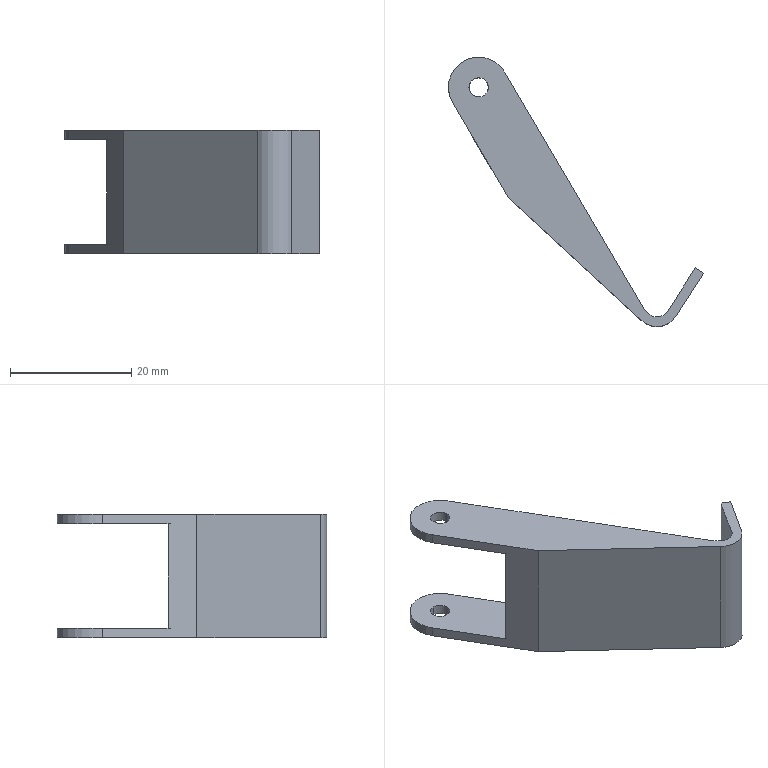Part | SolidWorks | features BaseBody 1 | 1 solid | 20 faces | box 42.12 x 44.482 x 20.4 mm | volume 2539 mm3 | plane 12 | cylinder 8 | commonest cylinder face diameters 3.2 x4 10 x2 4.14 x1 7.34 x1
STEP:
#1=CARTESIAN_POINT('',(2.549,31.982,8.6));
#2=VERTEX_POINT('',#1);
#3=CARTESIAN_POINT('',(-0.6512,31.982,8.6));
#4=VERTEX_POINT('',#3);
#5=CARTESIAN_POINT('',(0.9488,31.982,8.6));
#6=DIRECTION('',(0.,0.,-1.));
#7=DIRECTION('',(1.,0.,0.));
#8=AXIS2_PLACEMENT_3D('',#5,#6,#7);
#9=CIRCLE('',#8,1.6);
#10=EDGE_CURVE('',#2,#4,#9,.T.);
#11=ORIENTED_EDGE('',*,*,#10,.T.);
#12=CARTESIAN_POINT('',(-0.6512,31.982,10.2));
#13=VERTEX_POINT('',#12);
#14=CARTESIAN_POINT('',(-0.6512,31.982,8.6));
#15=DIRECTION('',(0.,0.,1.));
#16=VECTOR('',#15,1000.);
#17=LINE('',#14,#16);
#18=EDGE_CURVE('',#4,#13,#17,.T.);
#19=ORIENTED_EDGE('',*,*,#18,.T.);
#20=CARTESIAN_POINT('',(2.549,31.982,10.2));
#21=VERTEX_POINT('',#20);
#22=CARTESIAN_POINT('',(0.9488,31.982,10.2));
#23=DIRECTION('',(0.,0.,1.));
#24=DIRECTION('',(1.,0.,0.));
#25=AXIS2_PLACEMENT_3D('',#22,#23,#24);
#26=CIRCLE('',#25,1.6);
#27=EDGE_CURVE('',#13,#21,#26,.T.);
#28=ORIENTED_EDGE('',*,*,#27,.T.);
#29=CARTESIAN_POINT('',(2.549,31.982,8.6));
#30=DIRECTION('',(0.,0.,1.));
#31=VECTOR('',#30,1000.);
#32=LINE('',#29,#31);
#33=EDGE_CURVE('',#2,#21,#32,.T.);
#34=ORIENTED_EDGE('',*,*,#33,.F.);
#35=EDGE_LOOP('',(#11,#19,#28,#34));
#36=FACE_OUTER_BOUND('',#35,.T.);
#37=CARTESIAN_POINT('',(0.9488,31.982,8.6));
#38=DIRECTION('',(0.,0.,1.));
#39=DIRECTION('',(1.,0.,0.));
#40=AXIS2_PLACEMENT_3D('',#37,#38,#39);
#41=CYLINDRICAL_SURFACE('',#40,1.6);
#42=ADVANCED_FACE('',(#36),#41,.F.);
#43=CARTESIAN_POINT('',(0.9488,30.382,-10.2));
#44=VERTEX_POINT('',#43);
#45=CARTESIAN_POINT('',(0.9488,33.582,-10.2));
#46=VERTEX_POINT('',#45);
#47=CARTESIAN_POINT('',(0.9488,31.982,-10.2));
#48=DIRECTION('',(0.,0.,-1.));
#49=DIRECTION('',(0.,-1.,0.));
#50=AXIS2_PLACEMENT_3D('',#47,#48,#49);
#51=CIRCLE('',#50,1.6);
#52=EDGE_CURVE('',#44,#46,#51,.T.);
#53=ORIENTED_EDGE('',*,*,#52,.T.);
#54=CARTESIAN_POINT('',(0.9488,33.582,-8.6));
#55=VERTEX_POINT('',#54);
#56=CARTESIAN_POINT('',(0.9488,33.582,-10.2));
#57=DIRECTION('',(0.,0.,1.));
#58=VECTOR('',#57,1000.);
#59=LINE('',#56,#58);
#60=EDGE_CURVE('',#46,#55,#59,.T.);
#61=ORIENTED_EDGE('',*,*,#60,.T.);
#62=CARTESIAN_POINT('',(0.9488,30.382,-8.6));
#63=VERTEX_POINT('',#62);
#64=CARTESIAN_POINT('',(0.9488,31.982,-8.6));
#65=DIRECTION('',(0.,0.,1.));
#66=DIRECTION('',(0.,-1.,0.));
#67=AXIS2_PLACEMENT_3D('',#64,#65,#66);
#68=CIRCLE('',#67,1.6);
#69=EDGE_CURVE('',#55,#63,#68,.T.);
#70=ORIENTED_EDGE('',*,*,#69,.T.);
#71=CARTESIAN_POINT('',(0.9488,30.382,-10.2));
#72=DIRECTION('',(0.,0.,1.));
#73=VECTOR('',#72,1000.);
#74=LINE('',#71,#73);
#75=EDGE_CURVE('',#44,#63,#74,.T.);
#76=ORIENTED_EDGE('',*,*,#75,.F.);
#77=EDGE_LOOP('',(#53,#61,#70,#76));
#78=FACE_OUTER_BOUND('',#77,.T.);
#79=CARTESIAN_POINT('',(0.9488,31.982,-10.2));
#80=DIRECTION('',(0.,0.,1.));
#81=DIRECTION('',(0.,-1.,0.));
#82=AXIS2_PLACEMENT_3D('',#79,#80,#81);
#83=CYLINDRICAL_SURFACE('',#82,1.6);
#84=ADVANCED_FACE('',(#78),#83,.F.);
#85=ORIENTED_EDGE('',*,*,#18,.F.);
#86=CARTESIAN_POINT('',(0.9488,31.982,8.6));
#87=DIRECTION('',(0.,0.,-1.));
#88=DIRECTION('',(1.,0.,0.));
#89=AXIS2_PLACEMENT_3D('',#86,#87,#88);
#90=CIRCLE('',#89,1.6);
#91=EDGE_CURVE('',#4,#2,#90,.T.);
#92=ORIENTED_EDGE('',*,*,#91,.T.);
#93=ORIENTED_EDGE('',*,*,#33,.T.);
#94=CARTESIAN_POINT('',(0.9488,31.982,10.2));
#95=DIRECTION('',(0.,0.,1.));
#96=DIRECTION('',(1.,0.,0.));
#97=AXIS2_PLACEMENT_3D('',#94,#95,#96);
#98=CIRCLE('',#97,1.6);
#99=EDGE_CURVE('',#21,#13,#98,.T.);
#100=ORIENTED_EDGE('',*,*,#99,.T.);
#101=EDGE_LOOP('',(#85,#92,#93,#100));
#102=FACE_OUTER_BOUND('',#101,.T.);
#103=CARTESIAN_POINT('',(0.9488,31.982,8.6));
#104=DIRECTION('',(0.,0.,1.));
#105=DIRECTION('',(1.,0.,0.));
#106=AXIS2_PLACEMENT_3D('',#103,#104,#105);
#107=CYLINDRICAL_SURFACE('',#106,1.6);
#108=ADVANCED_FACE('',(#102),#107,.F.);
#109=ORIENTED_EDGE('',*,*,#99,.F.);
#110=ORIENTED_EDGE('',*,*,#27,.F.);
#111=EDGE_LOOP('',(#109,#110));
#112=FACE_BOUND('',#111,.T.);
#113=CARTESIAN_POINT('',(28.981,-5.35,10.2));
#114=VERTEX_POINT('',#113);
#115=CARTESIAN_POINT('',(32.127,-4.949,10.2));
#116=VERTEX_POINT('',#115);
#117=CARTESIAN_POINT('',(30.386,-3.83,10.2));
#118=DIRECTION('',(0.,0.,1.));
#119=DIRECTION('',(0.,1.,0.));
#120=AXIS2_PLACEMENT_3D('',#117,#118,#119);
#121=CIRCLE('',#120,2.07);
#122=EDGE_CURVE('',#114,#116,#121,.T.);
#123=ORIENTED_EDGE('',*,*,#122,.F.);
#124=CARTESIAN_POINT('',(28.303,-4.724,10.2));
#125=VERTEX_POINT('',#124);
#126=CARTESIAN_POINT('',(15.967,6.671,10.2));
#127=DIRECTION('',(-0.7345,0.6786,0.));
#128=VECTOR('',#127,1000.);
#129=LINE('',#126,#128);
#130=EDGE_CURVE('',#114,#125,#129,.T.);
#131=ORIENTED_EDGE('',*,*,#130,.T.);
#132=CARTESIAN_POINT('',(5.26,34.514,10.2));
#133=VERTEX_POINT('',#132);
#134=CARTESIAN_POINT('',(5.26,34.514,10.2));
#135=DIRECTION('',(0.5064,-0.8623,0.));
#136=VECTOR('',#135,1000.);
#137=LINE('',#134,#136);
#138=EDGE_CURVE('',#133,#125,#137,.T.);
#139=ORIENTED_EDGE('',*,*,#138,.F.);
#140=CARTESIAN_POINT('',(-3.363,29.45,10.2));
#141=VERTEX_POINT('',#140);
#142=CARTESIAN_POINT('',(0.9488,31.982,10.2));
#143=DIRECTION('',(0.,0.,-1.));
#144=DIRECTION('',(1.,0.,0.));
#145=AXIS2_PLACEMENT_3D('',#142,#143,#144);
#146=CIRCLE('',#145,5.);
#147=EDGE_CURVE('',#141,#133,#146,.T.);
#148=ORIENTED_EDGE('',*,*,#147,.F.);
#149=CARTESIAN_POINT('',(5.75,13.932,10.2));
#150=VERTEX_POINT('',#149);
#151=CARTESIAN_POINT('',(5.75,13.932,10.2));
#152=DIRECTION('',(-0.5064,0.8623,0.));
#153=VECTOR('',#152,1000.);
#154=LINE('',#151,#153);
#155=EDGE_CURVE('',#150,#141,#154,.T.);
#156=ORIENTED_EDGE('',*,*,#155,.F.);
#157=CARTESIAN_POINT('',(27.895,-6.526,10.2));
#158=VERTEX_POINT('',#157);
#159=CARTESIAN_POINT('',(5.75,13.932,10.2));
#160=DIRECTION('',(-0.7345,0.6786,0.));
#161=VECTOR('',#160,1000.);
#162=LINE('',#159,#161);
#163=EDGE_CURVE('',#158,#150,#162,.T.);
#164=ORIENTED_EDGE('',*,*,#163,.F.);
#165=CARTESIAN_POINT('',(33.473,-5.814,10.2));
#166=VERTEX_POINT('',#165);
#167=CARTESIAN_POINT('',(30.386,-3.83,10.2));
#168=DIRECTION('',(0.,0.,-1.));
#169=DIRECTION('',(0.,1.,0.));
#170=AXIS2_PLACEMENT_3D('',#167,#168,#169);
#171=CIRCLE('',#170,3.67);
#172=EDGE_CURVE('',#166,#158,#171,.T.);
#173=ORIENTED_EDGE('',*,*,#172,.F.);
#174=CARTESIAN_POINT('',(38.069,1.336,10.2));
#175=VERTEX_POINT('',#174);
#176=CARTESIAN_POINT('',(35.771,-2.239,10.2));
#177=DIRECTION('',(0.5407,0.8412,0.));
#178=VECTOR('',#177,1000.);
#179=LINE('',#176,#178);
#180=EDGE_CURVE('',#166,#175,#179,.T.);
#181=ORIENTED_EDGE('',*,*,#180,.T.);
#182=CARTESIAN_POINT('',(36.723,2.201,10.2));
#183=VERTEX_POINT('',#182);
#184=CARTESIAN_POINT('',(37.396,1.768,10.2));
#185=DIRECTION('',(0.8412,-0.5407,0.));
#186=VECTOR('',#185,1000.);
#187=LINE('',#184,#186);
#188=EDGE_CURVE('',#183,#175,#187,.T.);
#189=ORIENTED_EDGE('',*,*,#188,.F.);
#190=CARTESIAN_POINT('',(34.425,-1.374,10.2));
#191=DIRECTION('',(-0.5407,-0.8412,0.));
#192=VECTOR('',#191,1000.);
#193=LINE('',#190,#192);
#194=EDGE_CURVE('',#183,#116,#193,.T.);
#195=ORIENTED_EDGE('',*,*,#194,.T.);
#196=EDGE_LOOP('',(#123,#131,#139,#148,#156,#164,#173,#181,#189,#195));
#197=FACE_OUTER_BOUND('',#196,.T.);
#198=CARTESIAN_POINT('',(-4.276,-7.767,10.2));
#199=DIRECTION('',(0.,0.,-1.));
#200=DIRECTION('',(0.,1.,0.));
#201=AXIS2_PLACEMENT_3D('',#198,#199,#200);
#202=PLANE('',#201);
#203=ADVANCED_FACE('',(#112,#197),#202,.F.);
#204=ORIENTED_EDGE('',*,*,#10,.F.);
#205=ORIENTED_EDGE('',*,*,#91,.F.);
#206=EDGE_LOOP('',(#204,#205));
#207=FACE_BOUND('',#206,.T.);
#208=CARTESIAN_POINT('',(28.303,-4.724,8.6));
#209=VERTEX_POINT('',#208);
#210=CARTESIAN_POINT('',(5.26,34.514,8.6));
#211=VERTEX_POINT('',#210);
#212=CARTESIAN_POINT('',(5.26,34.514,8.6));
#213=DIRECTION('',(-0.5064,0.8623,0.));
#214=VECTOR('',#213,1000.);
#215=LINE('',#212,#214);
#216=EDGE_CURVE('',#209,#211,#215,.T.);
#217=ORIENTED_EDGE('',*,*,#216,.F.);
#218=CARTESIAN_POINT('',(2.954,18.693,8.6));
#219=VERTEX_POINT('',#218);
#220=CARTESIAN_POINT('',(9.94,12.24,8.6));
#221=DIRECTION('',(0.7345,-0.6786,0.));
#222=VECTOR('',#221,1000.);
#223=LINE('',#220,#222);
#224=EDGE_CURVE('',#219,#209,#223,.T.);
#225=ORIENTED_EDGE('',*,*,#224,.F.);
#226=CARTESIAN_POINT('',(-3.363,29.45,8.6));
#227=VERTEX_POINT('',#226);
#228=CARTESIAN_POINT('',(5.75,13.932,8.6));
#229=DIRECTION('',(0.5064,-0.8623,0.));
#230=VECTOR('',#229,1000.);
#231=LINE('',#228,#230);
#232=EDGE_CURVE('',#227,#219,#231,.T.);
#233=ORIENTED_EDGE('',*,*,#232,.F.);
#234=CARTESIAN_POINT('',(0.9488,31.982,8.6));
#235=DIRECTION('',(0.,0.,1.));
#236=DIRECTION('',(1.,0.,0.));
#237=AXIS2_PLACEMENT_3D('',#234,#235,#236);
#238=CIRCLE('',#237,5.);
#239=EDGE_CURVE('',#211,#227,#238,.T.);
#240=ORIENTED_EDGE('',*,*,#239,.F.);
#241=EDGE_LOOP('',(#217,#225,#233,#240));
#242=FACE_OUTER_BOUND('',#241,.T.);
#243=CARTESIAN_POINT('',(-8.644,29.408,8.6));
#244=DIRECTION('',(0.,0.,1.));
#245=DIRECTION('',(0.7345,-0.6786,0.));
#246=AXIS2_PLACEMENT_3D('',#243,#244,#245);
#247=PLANE('',#246);
#248=ADVANCED_FACE('',(#207,#242),#247,.F.);
#249=CARTESIAN_POINT('',(28.981,-5.35,-10.2));
#250=VERTEX_POINT('',#249);
#251=CARTESIAN_POINT('',(28.981,-5.35,0.));
#252=DIRECTION('',(0.,0.,1.));
#253=VECTOR('',#252,1000.);
#254=LINE('',#251,#253);
#255=EDGE_CURVE('',#250,#114,#254,.T.);
#256=ORIENTED_EDGE('',*,*,#255,.T.);
#257=ORIENTED_EDGE('',*,*,#122,.T.);
#258=CARTESIAN_POINT('',(32.127,-4.949,-10.2));
#259=VERTEX_POINT('',#258);
#260=CARTESIAN_POINT('',(32.127,-4.949,0.));
#261=DIRECTION('',(0.,0.,-1.));
#262=VECTOR('',#261,1000.);
#263=LINE('',#260,#262);
#264=EDGE_CURVE('',#116,#259,#263,.T.);
#265=ORIENTED_EDGE('',*,*,#264,.T.);
#266=CARTESIAN_POINT('',(30.386,-3.83,-10.2));
#267=DIRECTION('',(0.,0.,-1.));
#268=DIRECTION('',(0.,1.,0.));
#269=AXIS2_PLACEMENT_3D('',#266,#267,#268);
#270=CIRCLE('',#269,2.07);
#271=EDGE_CURVE('',#259,#250,#270,.T.);
#272=ORIENTED_EDGE('',*,*,#271,.T.);
#273=EDGE_LOOP('',(#256,#257,#265,#272));
#274=FACE_OUTER_BOUND('',#273,.T.);
#275=CARTESIAN_POINT('',(30.386,-3.83,10.2));
#276=DIRECTION('',(0.,0.,-1.));
#277=DIRECTION('',(0.,1.,0.));
#278=AXIS2_PLACEMENT_3D('',#275,#276,#277);
#279=CYLINDRICAL_SURFACE('',#278,2.07);
#280=ADVANCED_FACE('',(#274),#279,.F.);
#281=ORIENTED_EDGE('',*,*,#138,.T.);
#282=CARTESIAN_POINT('',(28.303,-4.724,9.4));
#283=DIRECTION('',(0.,0.,1.));
#284=VECTOR('',#283,1000.);
#285=LINE('',#282,#284);
#286=EDGE_CURVE('',#209,#125,#285,.T.);
#287=ORIENTED_EDGE('',*,*,#286,.F.);
#288=ORIENTED_EDGE('',*,*,#216,.T.);
#289=CARTESIAN_POINT('',(5.26,34.514,9.4));
#290=DIRECTION('',(0.,0.,-1.));
#291=VECTOR('',#290,1000.);
#292=LINE('',#289,#291);
#293=EDGE_CURVE('',#133,#211,#292,.T.);
#294=ORIENTED_EDGE('',*,*,#293,.F.);
#295=EDGE_LOOP('',(#281,#287,#288,#294));
#296=FACE_OUTER_BOUND('',#295,.T.);
#297=CARTESIAN_POINT('',(5.26,34.514,8.6));
#298=DIRECTION('',(-0.8623,-0.5064,0.));
#299=DIRECTION('',(0.5064,-0.8623,0.));
#300=AXIS2_PLACEMENT_3D('',#297,#298,#299);
#301=PLANE('',#300);
#302=ADVANCED_FACE('',(#296),#301,.F.);
#303=CARTESIAN_POINT('',(-3.363,29.45,9.4));
#304=DIRECTION('',(0.,0.,-1.));
#305=VECTOR('',#304,1000.);
#306=LINE('',#303,#305);
#307=EDGE_CURVE('',#141,#227,#306,.T.);
#308=ORIENTED_EDGE('',*,*,#307,.F.);
#309=ORIENTED_EDGE('',*,*,#147,.T.);
#310=ORIENTED_EDGE('',*,*,#293,.T.);
#311=ORIENTED_EDGE('',*,*,#239,.T.);
#312=EDGE_LOOP('',(#308,#309,#310,#311));
#313=FACE_OUTER_BOUND('',#312,.T.);
#314=CARTESIAN_POINT('',(0.9488,31.982,8.6));
#315=DIRECTION('',(0.,0.,1.));
#316=DIRECTION('',(1.,0.,0.));
#317=AXIS2_PLACEMENT_3D('',#314,#315,#316);
#318=CYLINDRICAL_SURFACE('',#317,5.);
#319=ADVANCED_FACE('',(#313),#318,.T.);
#320=ORIENTED_EDGE('',*,*,#307,.T.);
#321=ORIENTED_EDGE('',*,*,#232,.T.);
#322=CARTESIAN_POINT('',(2.954,18.693,-8.6));
#323=VERTEX_POINT('',#322);
#324=CARTESIAN_POINT('',(2.954,18.693,0.));
#325=DIRECTION('',(0.,0.,1.));
#326=VECTOR('',#325,1000.);
#327=LINE('',#324,#326);
#328=EDGE_CURVE('',#323,#219,#327,.T.);
#329=ORIENTED_EDGE('',*,*,#328,.F.);
#330=CARTESIAN_POINT('',(-3.363,29.45,-8.6));
#331=VERTEX_POINT('',#330);
#332=CARTESIAN_POINT('',(1.194,21.691,-8.6));
#333=DIRECTION('',(0.5064,-0.8623,0.));
#334=VECTOR('',#333,1000.);
#335=LINE('',#332,#334);
#336=EDGE_CURVE('',#331,#323,#335,.T.);
#337=ORIENTED_EDGE('',*,*,#336,.F.);
#338=CARTESIAN_POINT('',(-3.363,29.45,-10.2));
#339=VERTEX_POINT('',#338);
#340=CARTESIAN_POINT('',(-3.363,29.45,-9.4));
#341=DIRECTION('',(0.,0.,-1.));
#342=VECTOR('',#341,1000.);
#343=LINE('',#340,#342);
#344=EDGE_CURVE('',#331,#339,#343,.T.);
#345=ORIENTED_EDGE('',*,*,#344,.T.);
#346=CARTESIAN_POINT('',(5.75,13.932,-10.2));
#347=VERTEX_POINT('',#346);
#348=CARTESIAN_POINT('',(1.194,21.691,-10.2));
#349=DIRECTION('',(-0.5064,0.8623,0.));
#350=VECTOR('',#349,1000.);
#351=LINE('',#348,#350);
#352=EDGE_CURVE('',#347,#339,#351,.T.);
#353=ORIENTED_EDGE('',*,*,#352,.F.);
#354=CARTESIAN_POINT('',(5.75,13.932,0.));
#355=DIRECTION('',(0.,0.,-1.));
#356=VECTOR('',#355,1000.);
#357=LINE('',#354,#356);
#358=EDGE_CURVE('',#150,#347,#357,.T.);
#359=ORIENTED_EDGE('',*,*,#358,.F.);
#360=ORIENTED_EDGE('',*,*,#155,.T.);
#361=EDGE_LOOP('',(#320,#321,#329,#337,#345,#353,#359,#360));
#362=FACE_OUTER_BOUND('',#361,.T.);
#363=CARTESIAN_POINT('',(5.75,13.932,-10.2));
#364=DIRECTION('',(0.8623,0.5064,0.));
#365=DIRECTION('',(-0.5064,0.8623,0.));
#366=AXIS2_PLACEMENT_3D('',#363,#364,#365);
#367=PLANE('',#366);
#368=ADVANCED_FACE('',(#362),#367,.F.);
#369=ORIENTED_EDGE('',*,*,#163,.T.);
#370=ORIENTED_EDGE('',*,*,#358,.T.);
#371=CARTESIAN_POINT('',(27.895,-6.526,-10.2));
#372=VERTEX_POINT('',#371);
#373=CARTESIAN_POINT('',(16.823,3.703,-10.2));
#374=DIRECTION('',(-0.7345,0.6786,0.));
#375=VECTOR('',#374,1000.);
#376=LINE('',#373,#375);
#377=EDGE_CURVE('',#372,#347,#376,.T.);
#378=ORIENTED_EDGE('',*,*,#377,.F.);
#379=CARTESIAN_POINT('',(27.895,-6.526,0.));
#380=DIRECTION('',(0.,0.,-1.));
#381=VECTOR('',#380,1000.);
#382=LINE('',#379,#381);
#383=EDGE_CURVE('',#158,#372,#382,.T.);
#384=ORIENTED_EDGE('',*,*,#383,.F.);
#385=EDGE_LOOP('',(#369,#370,#378,#384));
#386=FACE_OUTER_BOUND('',#385,.T.);
#387=CARTESIAN_POINT('',(5.75,13.932,-10.2));
#388=DIRECTION('',(0.6786,0.7345,0.));
#389=DIRECTION('',(0.,0.,1.));
#390=AXIS2_PLACEMENT_3D('',#387,#388,#389);
#391=PLANE('',#390);
#392=ADVANCED_FACE('',(#386),#391,.F.);
#393=ORIENTED_EDGE('',*,*,#172,.T.);
#394=ORIENTED_EDGE('',*,*,#383,.T.);
#395=CARTESIAN_POINT('',(33.473,-5.814,-10.2));
#396=VERTEX_POINT('',#395);
#397=CARTESIAN_POINT('',(30.386,-3.83,-10.2));
#398=DIRECTION('',(0.,0.,-1.));
#399=DIRECTION('',(0.,1.,0.));
#400=AXIS2_PLACEMENT_3D('',#397,#398,#399);
#401=CIRCLE('',#400,3.67);
#402=EDGE_CURVE('',#396,#372,#401,.T.);
#403=ORIENTED_EDGE('',*,*,#402,.F.);
#404=CARTESIAN_POINT('',(33.473,-5.814,0.));
#405=DIRECTION('',(0.,0.,-1.));
#406=VECTOR('',#405,1000.);
#407=LINE('',#404,#406);
#408=EDGE_CURVE('',#166,#396,#407,.T.);
#409=ORIENTED_EDGE('',*,*,#408,.F.);
#410=EDGE_LOOP('',(#393,#394,#403,#409));
#411=FACE_OUTER_BOUND('',#410,.T.);
#412=CARTESIAN_POINT('',(30.386,-3.83,10.2));
#413=DIRECTION('',(0.,0.,-1.));
#414=DIRECTION('',(0.,1.,0.));
#415=AXIS2_PLACEMENT_3D('',#412,#413,#414);
#416=CYLINDRICAL_SURFACE('',#415,3.67);
#417=ADVANCED_FACE('',(#411),#416,.T.);
#418=CARTESIAN_POINT('',(28.303,-4.724,-10.2));
#419=VERTEX_POINT('',#418);
#420=CARTESIAN_POINT('',(15.967,6.671,-10.2));
#421=DIRECTION('',(0.7345,-0.6786,0.));
#422=VECTOR('',#421,1000.);
#423=LINE('',#420,#422);
#424=EDGE_CURVE('',#419,#250,#423,.T.);
#425=ORIENTED_EDGE('',*,*,#424,.F.);
#426=CARTESIAN_POINT('',(28.303,-4.724,-8.6));
#427=VERTEX_POINT('',#426);
#428=CARTESIAN_POINT('',(28.303,-4.724,-9.4));
#429=DIRECTION('',(0.,0.,1.));
#430=VECTOR('',#429,1000.);
#431=LINE('',#428,#430);
#432=EDGE_CURVE('',#419,#427,#431,.T.);
#433=ORIENTED_EDGE('',*,*,#432,.T.);
#434=CARTESIAN_POINT('',(15.967,6.671,-8.6));
#435=DIRECTION('',(0.7345,-0.6786,0.));
#436=VECTOR('',#435,1000.);
#437=LINE('',#434,#436);
#438=EDGE_CURVE('',#323,#427,#437,.T.);
#439=ORIENTED_EDGE('',*,*,#438,.F.);
#440=ORIENTED_EDGE('',*,*,#328,.T.);
#441=ORIENTED_EDGE('',*,*,#224,.T.);
#442=ORIENTED_EDGE('',*,*,#286,.T.);
#443=ORIENTED_EDGE('',*,*,#130,.F.);
#444=ORIENTED_EDGE('',*,*,#255,.F.);
#445=EDGE_LOOP('',(#425,#433,#439,#440,#441,#442,#443,#444));
#446=FACE_OUTER_BOUND('',#445,.T.);
#447=CARTESIAN_POINT('',(2.954,18.693,10.2));
#448=DIRECTION('',(-0.6786,-0.7345,0.));
#449=DIRECTION('',(0.,0.,-1.));
#450=AXIS2_PLACEMENT_3D('',#447,#448,#449);
#451=PLANE('',#450);
#452=ADVANCED_FACE('',(#446),#451,.F.);
#453=ORIENTED_EDGE('',*,*,#52,.F.);
#454=CARTESIAN_POINT('',(0.9488,31.982,-10.2));
#455=DIRECTION('',(0.,0.,-1.));
#456=DIRECTION('',(0.,-1.,0.));
#457=AXIS2_PLACEMENT_3D('',#454,#455,#456);
#458=CIRCLE('',#457,1.6);
#459=EDGE_CURVE('',#46,#44,#458,.T.);
#460=ORIENTED_EDGE('',*,*,#459,.F.);
#461=EDGE_LOOP('',(#453,#460));
#462=FACE_BOUND('',#461,.T.);
#463=ORIENTED_EDGE('',*,*,#402,.T.);
#464=ORIENTED_EDGE('',*,*,#377,.T.);
#465=ORIENTED_EDGE('',*,*,#352,.T.);
#466=CARTESIAN_POINT('',(5.26,34.514,-10.2));
#467=VERTEX_POINT('',#466);
#468=CARTESIAN_POINT('',(0.9488,31.982,-10.2));
#469=DIRECTION('',(0.,0.,1.));
#470=DIRECTION('',(0.,-1.,0.));
#471=AXIS2_PLACEMENT_3D('',#468,#469,#470);
#472=CIRCLE('',#471,5.);
#473=EDGE_CURVE('',#467,#339,#472,.T.);
#474=ORIENTED_EDGE('',*,*,#473,.F.);
#475=CARTESIAN_POINT('',(5.26,34.514,-10.2));
#476=DIRECTION('',(-0.5064,0.8623,0.));
#477=VECTOR('',#476,1000.);
#478=LINE('',#475,#477);
#479=EDGE_CURVE('',#419,#467,#478,.T.);
#480=ORIENTED_EDGE('',*,*,#479,.F.);
#481=ORIENTED_EDGE('',*,*,#424,.T.);
#482=ORIENTED_EDGE('',*,*,#271,.F.);
#483=CARTESIAN_POINT('',(36.723,2.201,-10.2));
#484=VERTEX_POINT('',#483);
#485=CARTESIAN_POINT('',(36.328,1.586,-10.2));
#486=DIRECTION('',(-0.5407,-0.8412,0.));
#487=VECTOR('',#486,1000.);
#488=LINE('',#485,#487);
#489=EDGE_CURVE('',#484,#259,#488,.T.);
#490=ORIENTED_EDGE('',*,*,#489,.F.);
#491=CARTESIAN_POINT('',(38.069,1.336,-10.2));
#492=VERTEX_POINT('',#491);
#493=CARTESIAN_POINT('',(37.396,1.768,-10.2));
#494=DIRECTION('',(0.8412,-0.5407,0.));
#495=VECTOR('',#494,1000.);
#496=LINE('',#493,#495);
#497=EDGE_CURVE('',#484,#492,#496,.T.);
#498=ORIENTED_EDGE('',*,*,#497,.T.);
#499=CARTESIAN_POINT('',(37.674,0.7211,-10.2));
#500=DIRECTION('',(0.5407,0.8412,0.));
#501=VECTOR('',#500,1000.);
#502=LINE('',#499,#501);
#503=EDGE_CURVE('',#396,#492,#502,.T.);
#504=ORIENTED_EDGE('',*,*,#503,.F.);
#505=EDGE_LOOP('',(#463,#464,#465,#474,#480,#481,#482,#490,#498,#504));
#506=FACE_OUTER_BOUND('',#505,.T.);
#507=CARTESIAN_POINT('',(31.414,-9.017,-10.2));
#508=DIRECTION('',(0.,0.,1.));
#509=DIRECTION('',(0.5407,0.8412,0.));
#510=AXIS2_PLACEMENT_3D('',#507,#508,#509);
#511=PLANE('',#510);
#512=ADVANCED_FACE('',(#462,#506),#511,.F.);
#513=ORIENTED_EDGE('',*,*,#264,.F.);
#514=ORIENTED_EDGE('',*,*,#194,.F.);
#515=CARTESIAN_POINT('',(36.723,2.201,0.));
#516=DIRECTION('',(0.,0.,1.));
#517=VECTOR('',#516,1000.);
#518=LINE('',#515,#517);
#519=EDGE_CURVE('',#484,#183,#518,.T.);
#520=ORIENTED_EDGE('',*,*,#519,.F.);
#521=ORIENTED_EDGE('',*,*,#489,.T.);
#522=EDGE_LOOP('',(#513,#514,#520,#521));
#523=FACE_OUTER_BOUND('',#522,.T.);
#524=CARTESIAN_POINT('',(32.127,-4.949,10.2));
#525=DIRECTION('',(0.8412,-0.5407,0.));
#526=DIRECTION('',(0.,0.,-1.));
#527=AXIS2_PLACEMENT_3D('',#524,#525,#526);
#528=PLANE('',#527);
#529=ADVANCED_FACE('',(#523),#528,.F.);
#530=CARTESIAN_POINT('',(0.9488,31.982,-8.6));
#531=DIRECTION('',(0.,0.,1.));
#532=DIRECTION('',(0.,-1.,0.));
#533=AXIS2_PLACEMENT_3D('',#530,#531,#532);
#534=CIRCLE('',#533,1.6);
#535=EDGE_CURVE('',#63,#55,#534,.T.);
#536=ORIENTED_EDGE('',*,*,#535,.F.);
#537=ORIENTED_EDGE('',*,*,#69,.F.);
#538=EDGE_LOOP('',(#536,#537));
#539=FACE_BOUND('',#538,.T.);
#540=CARTESIAN_POINT('',(5.26,34.514,-8.6));
#541=VERTEX_POINT('',#540);
#542=CARTESIAN_POINT('',(5.26,34.514,-8.6));
#543=DIRECTION('',(0.5064,-0.8623,0.));
#544=VECTOR('',#543,1000.);
#545=LINE('',#542,#544);
#546=EDGE_CURVE('',#541,#427,#545,.T.);
#547=ORIENTED_EDGE('',*,*,#546,.F.);
#548=CARTESIAN_POINT('',(0.9488,31.982,-8.6));
#549=DIRECTION('',(0.,0.,-1.));
#550=DIRECTION('',(0.,-1.,0.));
#551=AXIS2_PLACEMENT_3D('',#548,#549,#550);
#552=CIRCLE('',#551,5.);
#553=EDGE_CURVE('',#331,#541,#552,.T.);
#554=ORIENTED_EDGE('',*,*,#553,.F.);
#555=ORIENTED_EDGE('',*,*,#336,.T.);
#556=ORIENTED_EDGE('',*,*,#438,.T.);
#557=EDGE_LOOP('',(#547,#554,#555,#556));
#558=FACE_OUTER_BOUND('',#557,.T.);
#559=CARTESIAN_POINT('',(28.523,-4.928,-8.6));
#560=DIRECTION('',(0.,0.,-1.));
#561=DIRECTION('',(-0.7345,0.6786,0.));
#562=AXIS2_PLACEMENT_3D('',#559,#560,#561);
#563=PLANE('',#562);
#564=ADVANCED_FACE('',(#539,#558),#563,.F.);
#565=ORIENTED_EDGE('',*,*,#408,.T.);
#566=ORIENTED_EDGE('',*,*,#503,.T.);
#567=CARTESIAN_POINT('',(38.069,1.336,0.));
#568=DIRECTION('',(0.,0.,-1.));
#569=VECTOR('',#568,1000.);
#570=LINE('',#567,#569);
#571=EDGE_CURVE('',#175,#492,#570,.T.);
#572=ORIENTED_EDGE('',*,*,#571,.F.);
#573=ORIENTED_EDGE('',*,*,#180,.F.);
#574=EDGE_LOOP('',(#565,#566,#572,#573));
#575=FACE_OUTER_BOUND('',#574,.T.);
#576=CARTESIAN_POINT('',(33.473,-5.814,-10.2));
#577=DIRECTION('',(-0.8412,0.5407,0.));
#578=DIRECTION('',(0.,0.,1.));
#579=AXIS2_PLACEMENT_3D('',#576,#577,#578);
#580=PLANE('',#579);
#581=ADVANCED_FACE('',(#575),#580,.F.);
#582=ORIENTED_EDGE('',*,*,#60,.F.);
#583=ORIENTED_EDGE('',*,*,#459,.T.);
#584=ORIENTED_EDGE('',*,*,#75,.T.);
#585=ORIENTED_EDGE('',*,*,#535,.T.);
#586=EDGE_LOOP('',(#582,#583,#584,#585));
#587=FACE_OUTER_BOUND('',#586,.T.);
#588=CARTESIAN_POINT('',(0.9488,31.982,-10.2));
#589=DIRECTION('',(0.,0.,1.));
#590=DIRECTION('',(0.,-1.,0.));
#591=AXIS2_PLACEMENT_3D('',#588,#589,#590);
#592=CYLINDRICAL_SURFACE('',#591,1.6);
#593=ADVANCED_FACE('',(#587),#592,.F.);
#594=ORIENTED_EDGE('',*,*,#344,.F.);
#595=ORIENTED_EDGE('',*,*,#553,.T.);
#596=CARTESIAN_POINT('',(5.26,34.514,-9.4));
#597=DIRECTION('',(0.,0.,1.));
#598=VECTOR('',#597,1000.);
#599=LINE('',#596,#598);
#600=EDGE_CURVE('',#467,#541,#599,.T.);
#601=ORIENTED_EDGE('',*,*,#600,.F.);
#602=ORIENTED_EDGE('',*,*,#473,.T.);
#603=EDGE_LOOP('',(#594,#595,#601,#602));
#604=FACE_OUTER_BOUND('',#603,.T.);
#605=CARTESIAN_POINT('',(0.9488,31.982,-10.2));
#606=DIRECTION('',(0.,0.,1.));
#607=DIRECTION('',(0.,-1.,0.));
#608=AXIS2_PLACEMENT_3D('',#605,#606,#607);
#609=CYLINDRICAL_SURFACE('',#608,5.);
#610=ADVANCED_FACE('',(#604),#609,.T.);
#611=ORIENTED_EDGE('',*,*,#546,.T.);
#612=ORIENTED_EDGE('',*,*,#432,.F.);
#613=ORIENTED_EDGE('',*,*,#479,.T.);
#614=ORIENTED_EDGE('',*,*,#600,.T.);
#615=EDGE_LOOP('',(#611,#612,#613,#614));
#616=FACE_OUTER_BOUND('',#615,.T.);
#617=CARTESIAN_POINT('',(5.26,34.514,-10.2));
#618=DIRECTION('',(-0.8623,-0.5064,0.));
#619=DIRECTION('',(0.5064,-0.8623,0.));
#620=AXIS2_PLACEMENT_3D('',#617,#618,#619);
#621=PLANE('',#620);
#622=ADVANCED_FACE('',(#616),#621,.F.);
#623=ORIENTED_EDGE('',*,*,#519,.T.);
#624=ORIENTED_EDGE('',*,*,#188,.T.);
#625=ORIENTED_EDGE('',*,*,#571,.T.);
#626=ORIENTED_EDGE('',*,*,#497,.F.);
#627=EDGE_LOOP('',(#623,#624,#625,#626));
#628=FACE_OUTER_BOUND('',#627,.T.);
#629=CARTESIAN_POINT('',(38.069,1.336,-10.2));
#630=DIRECTION('',(-0.5407,-0.8412,0.));
#631=DIRECTION('',(0.,0.,1.));
#632=AXIS2_PLACEMENT_3D('',#629,#630,#631);
#633=PLANE('',#632);
#634=ADVANCED_FACE('',(#628),#633,.F.);
#635=CLOSED_SHELL('',(#42,#84,#108,#203,#248,#280,#302,#319,#368,#392,#417,#452,#512,#529,#564,#581,#593,#610,#622,#634));
#636=MANIFOLD_SOLID_BREP('',#635);
#637=CARTESIAN_POINT('',(0.,0.,0.));
#638=DIRECTION('',(0.,0.,1.));
#639=DIRECTION('',(1.,0.,0.));
#640=AXIS2_PLACEMENT_3D('',#637,#638,#639);
#641=(LENGTH_UNIT()NAMED_UNIT(*)SI_UNIT(.MILLI.,.METRE.));
#642=UNCERTAINTY_MEASURE_WITH_UNIT(LENGTH_MEASURE(0.00001),#641,'','');
#643=(NAMED_UNIT(*)PLANE_ANGLE_UNIT()SI_UNIT($,.RADIAN.));
#644=(NAMED_UNIT(*)SI_UNIT($,.STERADIAN.)SOLID_ANGLE_UNIT());
#645=(GEOMETRIC_REPRESENTATION_CONTEXT(3)GLOBAL_UNCERTAINTY_ASSIGNED_CONTEXT((#642))GLOBAL_UNIT_ASSIGNED_CONTEXT((#641,#643,#644))REPRESENTATION_CONTEXT('',''));
#646=ADVANCED_BREP_SHAPE_REPRESENTATION('',(#636,#640),#645);